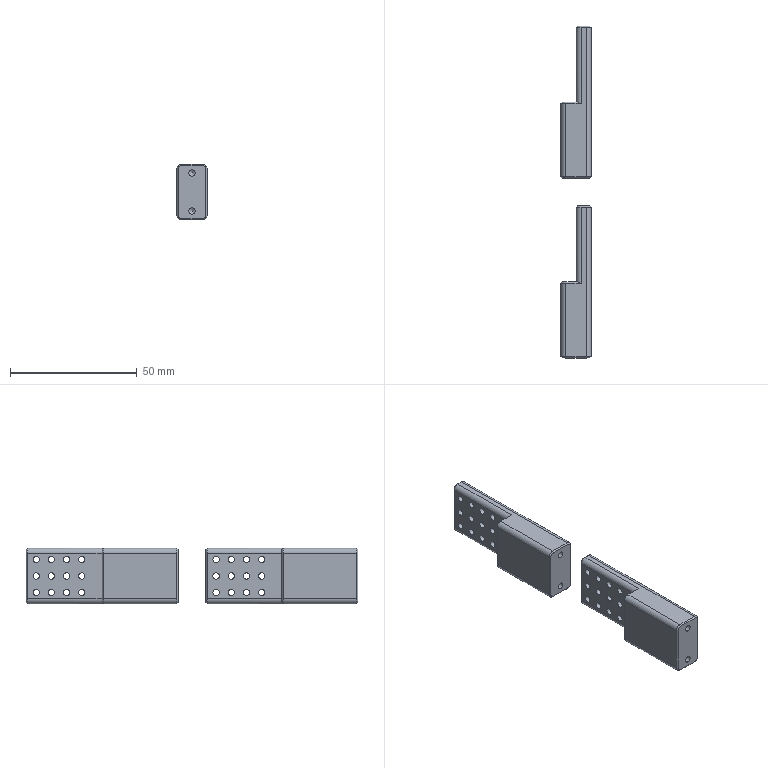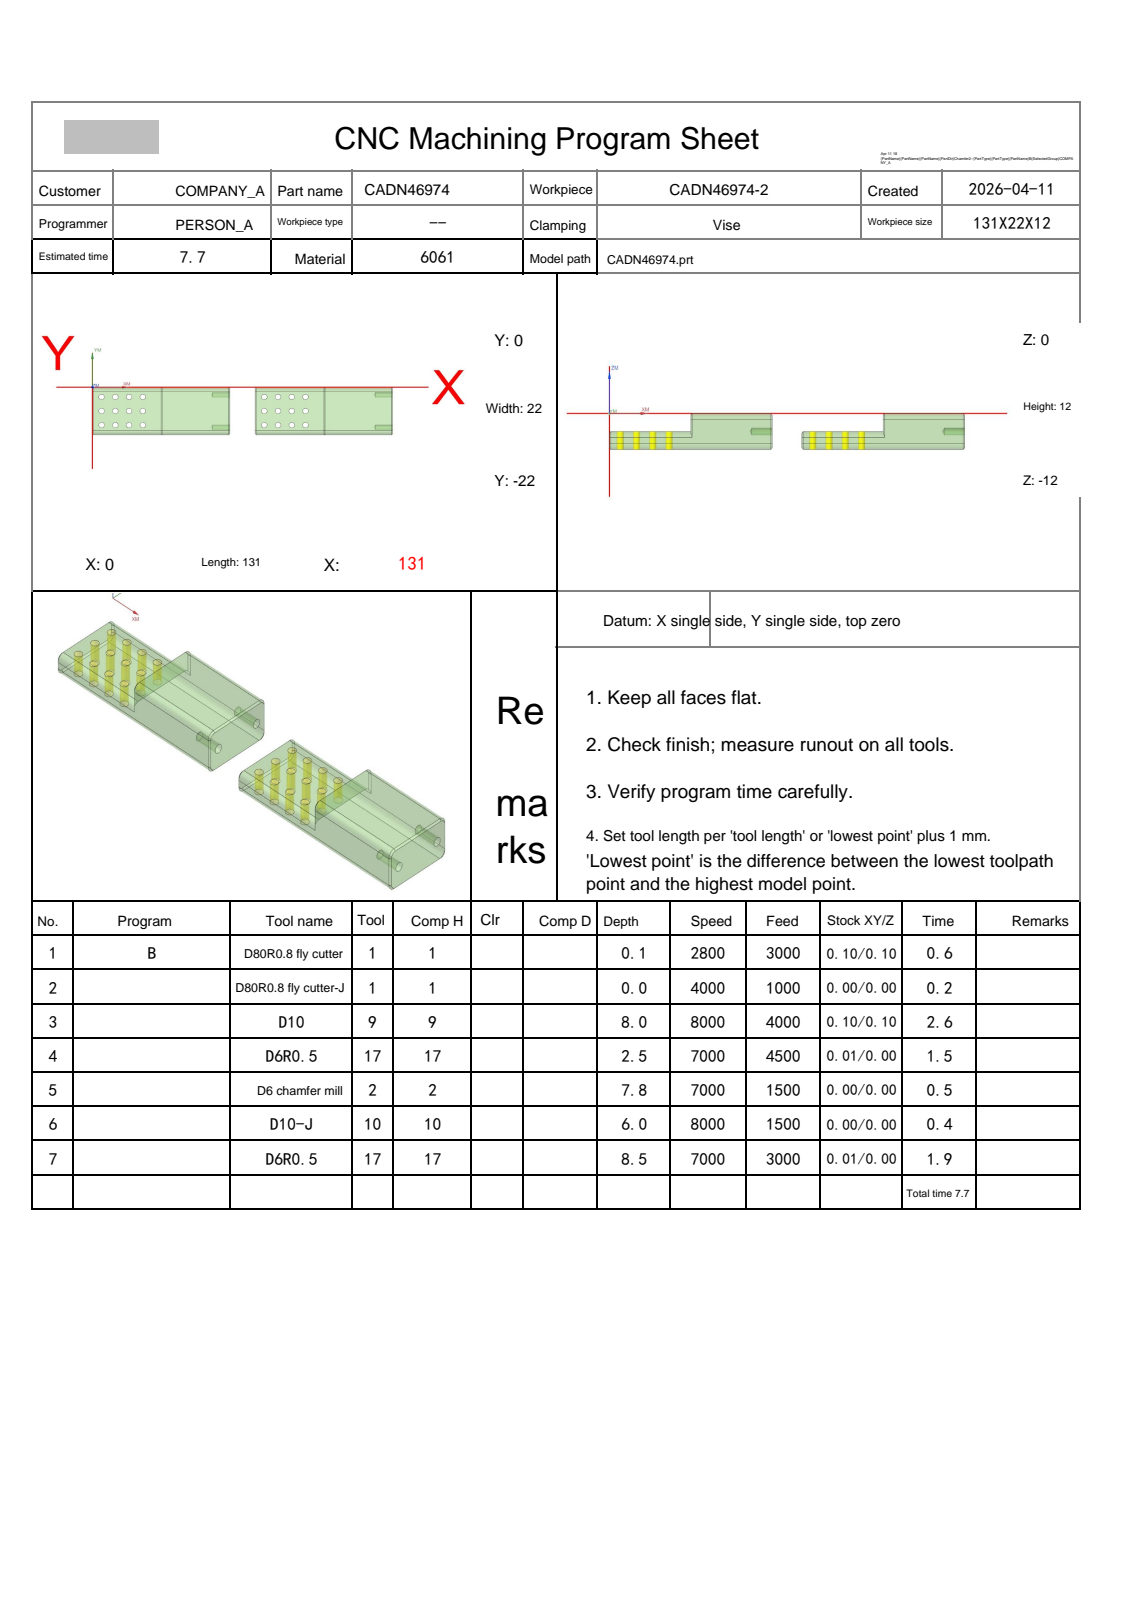NC program | NX | posted by the shop | part box 12 x 131 x 22 mm
Lines 1 to 2207 of 5054, first 1773 of 2205 lines:
%
O0001
(Machine time: 9.04 MIN)
(===Total Tool:5===)
(T1=D80R0.8 fly cutter D=80.  R=0.8  D-  H01 Z=0.    )
(T9=D10     D=10.  R=0.   D-  H09 Z=-8.   )
(T17=D6R0.5 D=6.   R=0.5  D-  H17 Z=-8.5  )
(T2=D6 chamfer mill   D=6.   R=0.   D-  H02 Z=-7.75 )
(T10=D10-J  D=10.  R=0.   D10 H10 Z=-6.   )
G80 G90 G17 G49 G40
G91 G28 Z0
M01
N1 T01 M06
(D80R0.8 fly cutter  D=80. R=0.8 H=01 ce=0.10 di=0.10)
G00 G90 G54 X183.097 Y-11. M03 S2800
G43 H01 Z20.
M08
Z4.517
G01 Z2.517 F3000.
X171.097
X-40.097
X-52.097
Z4.517
G00 X183.097
Z4.033
G01 Z2.033
X171.097
X-40.097
X-52.097
Z4.033
G00 X183.097
Z3.55
G01 Z1.55
X171.097
X-40.097
X-52.097
Z3.55
G00 X183.097
Z3.067
G01 Z1.067
X171.097
X-40.097
X-52.097
Z3.067
G00 Z20.
X183.097
Z2.583
G01 Z.583
X171.097
X-40.097
X-52.097
Z2.583
G00 Z20.
X183.097
Z2.1
G01 Z.1
X171.097
X-40.097
X-52.097
Z2.1
G00 Z20.
G91 G28 Z0.0
M05
M09
G91 G28 Z0.0
M01
N2 T01 M06
(D80R0.8 fly cutter-J  D=80. R=0.8 H=01 ce=0.00 di=0.00)
G00 G90 G54 X182.999 Y-11. M03 S4000
G43 H01 Z20.
M08
Z2.
G01 Z0.0 F1000.
X170.999
X-39.999
X-51.999
Z2.
G00 Z20.
G91 G28 Z0.0
M05
M09
G91 G28 Z0.0
M01
N3 T09 M06
(D10  D=10. R=0. H=09 ce=0.10 di=0.10)
G00 G90 G54 X18.201 Y-34.02 M03 S8000
G43 H09 Z12.8
M08
Z.708
G01 Z-.492 F4000.
Y-31.
G03 X11.201 Y-24. I-7. J0.0
G01 X4.502
X-1.996
X-1.999
G02 X-2.498 Y-23.507 I0.0 J.499
G01 X-2.5 Y1.507
G02 X-1.999 Y2.001 I.501 J-.006
G01 X-1.964 Y2.
X24.507
G02 X25.997 Y4.005 I7.492 J-4.012
X27.326 Y5.02 I4.489 J-4.5
G01 X58.797
X59.246
X59.378 Y5.022
G02 X63.361 Y3.238 I0.0 J-5.341
X64.059 Y2. I-8.104 J-5.382
X64.589 Y.608 I-8.801 J-4.144
G01 X64.591 Y.601
G03 X64.044 Y1.653 I-6.299 J-2.603
G01 X63.713 Y2.198
G03 X59.5 Y4.461 I-4.266 J-2.888
G01 X30.486
G03 X26.985 Y3.014 I0.0 J-4.956
X24.9 Y-2.001 I5.013 J-5.025
G01 Y-19.999
Y-20.028
G03 X26.176 Y-24.037 I6.936 J0.0
G01 X26.539 Y-24.526
G03 X30.5 Y-26.461 I4.015 J3.195
G01 X59.5
G03 X63.713 Y-24.198 I-.053 J5.151
X64.59 Y-22.581 I-6.897 J4.786
G01 X64.588 Y-22.587
X64.53 Y-22.798
X64.239 Y-23.627
G02 X64.095 Y-24. I-4.741 J1.615
X59.5 Y-27.02 I-4.597 J1.988
G01 X30.366
X29.131
X28.858
X27.348
G02 X25.416 Y-25.361 I3.208 J5.689
G01 X25.034 Y-24.847
G02 X24.507 Y-24. I6.803 J4.819
G01 X6.201
G02 X5.201 Y-23. I0.0 J1.
G01 X5.202 Y-22.95
X5.461 Y-17.759
X5.463 Y-17.709
G03 X4.982 Y-16.855 I-1. J0.0
G02 X4.501 Y-16.002 I.519 J.855
G01 Y-5.998
G02 X5.498 Y-5. I1. J-.002
G01 X16.903
G02 X17.9 Y-5.998 I-.002 J-1.
G01 Y-16.002
G02 X16.903 Y-17. I-1. J.002
G01 X9.643
G02 X8.743 Y-16.1 I0.0 J.9
G01 X8.744 Y-16.059
X9. Y-10.515
X9.001 Y-10.485
G02 X9.999 Y-9.5 I1. J-.015
G01 X12.403
G02 X13.4 Y-10.498 I-.002 J-1.
G01 Y-11.502
G02 X12.403 Y-12.5 I-1. J.002
G01 X9.999
G02 X9.433 Y-12.323 I.002 J1.
X9.108 Y-11.949 I.568 J.823
G03 X2.855 Y-8.096 I-6.253 J-3.146
X-.292 Y-8.843 I0.0 J-7.
G01 X-11.991 Y-14.729
Z.708
G00 Z3.
G01 X18.201 Y-34.18 F6000.
G00 Z.217
G01 Z-.983 F4000.
Y-31.
G03 X11.201 Y-24. I-7. J0.0
G01 X4.502
X-1.996
X-1.999
G02 X-2.498 Y-23.507 I0.0 J.499
G01 X-2.5 Y1.507
G02 X-1.999 Y2.001 I.501 J-.006
G01 X-1.964 Y2.
X24.18
G02 X25.066 Y3.361 I5.999 J-2.937
X26.976 Y5.18 I5.552 J-3.917
G01 X58.797
X59.243
X59.376 Y5.182
G02 X63.492 Y3.331 I0.0 J-5.501
X64.19 Y2.098 I-8.234 J-5.475
G01 X64.136 Y2.058
X64.082 Y2.13
G03 X63.042 Y3.398 I-6.938 J-4.629
X59.5 Y4.837 I-3.583 J-3.74
G01 X30.5
G03 X26.176 Y2.505 I.119 J-5.394
X24.9 Y-.898 I4.003 J-3.442
G01 Y-21.102
G03 X26.176 Y-24.505 I5.279 J.039
X30.5 Y-26.837 I4.442 J3.061
G01 X59.507
G03 X63.003 Y-25.429 I0.0 J5.044
X64.082 Y-24.13 I-5.234 J5.443
G01 X64.136 Y-24.058
X64.218 Y-24.118
G02 X59.5 Y-27.18 I-4.72 J2.106
G01 X30.366
X29.131
X28.858
X26.976
G02 X25.066 Y-25.361 I3.642 J5.736
X24.18 Y-24. I5.113 J4.298
G01 X6.201
G02 X5.201 Y-23. I0.0 J1.
G01 X5.202 Y-22.95
X5.461 Y-17.759
X5.462 Y-17.709
G03 X4.982 Y-16.855 I-1. J0.0
G02 X4.501 Y-16.002 I.519 J.855
G01 Y-5.998
G02 X5.498 Y-5. I1. J-.002
G01 X16.902
G02 X17.9 Y-5.998 I-.002 J-1.
G01 Y-16.002
G02 X16.902 Y-17. I-1. J.002
G01 X9.643
G02 X8.743 Y-16.1 I0.0 J.9
G01 X8.744 Y-16.059
X9. Y-10.515
X9.001 Y-10.485
G02 X9.999 Y-9.5 I1. J-.015
G01 X12.402
G02 X13.4 Y-10.498 I-.002 J-1.
G01 Y-11.502
G02 X12.402 Y-12.5 I-1. J.002
G01 X9.999
G02 X9.433 Y-12.323 I.002 J1.
X9.108 Y-11.949 I.568 J.823
G03 X2.855 Y-8.095 I-6.253 J-3.146
X-.291 Y-8.842 I0.0 J-7.
G01 X-12.151 Y-14.809
Z.217
G00 Z2.508
G01 X18.201 Y-34.18 F6000.
G00 Z-.275
G01 Z-1.475 F4000.
Y-31.
G03 X11.201 Y-24. I-7. J0.0
G01 X4.502
X-1.996
X-1.999
G02 X-2.498 Y-23.507 I0.0 J.499
G01 X-2.5 Y1.507
G02 X-1.999 Y2.001 I.501 J-.006
G01 X-1.964 Y2.
X24.052
G02 X25.413 Y3.995 I6.003 J-2.634
X26.688 Y5.18 I5.194 J-4.31
G01 X58.797
X59.243
X59.376 Y5.182
G02 X63.492 Y3.331 I0.0 J-5.501
X63.759 Y2.906 I-8.234 J-5.475
G01 X63.73 Y2.879
X63.222 Y3.398
G03 X59.5 Y5.033 I-3.748 J-3.477
G01 X30.5
G03 X26.45 Y3.052 I.107 J-5.348
X24.9 Y-.591 I3.605 J-3.685
G01 Y-21.409
G03 X26.45 Y-25.052 I5.155 J.043
X30.5 Y-27.033 I4.153 J3.358
G01 X59.5
G03 X63.222 Y-25.398 I-.025 J5.112
G01 X63.717 Y-24.892
X63.76 Y-24.934
G02 X59.5 Y-27.18 I-4.263 J2.922
G01 X30.366
X29.131
X28.858
X26.687
G02 X25.413 Y-25.995 I3.916 J5.486
X24.052 Y-24. I4.642 J4.629
G01 X6.201
G02 X5.201 Y-23. I0.0 J1.
G01 X5.202 Y-22.95
X5.461 Y-17.759
X5.462 Y-17.709
G03 X4.982 Y-16.855 I-1. J0.0
G02 X4.501 Y-16.002 I.519 J.855
G01 Y-5.998
G02 X5.498 Y-5. I1. J-.002
G01 X16.902
G02 X17.9 Y-5.998 I-.002 J-1.
G01 Y-16.002
G02 X16.902 Y-17. I-1. J.002
G01 X9.643
G02 X8.743 Y-16.1 I0.0 J.9
G01 X8.744 Y-16.059
X9. Y-10.515
X9.001 Y-10.485
G02 X9.998 Y-9.5 I1. J-.015
G01 X12.403
G02 X13.4 Y-10.497 I-.003 J-1.
G01 Y-11.503
G02 X12.403 Y-12.5 I-1. J.003
G01 X9.999
G02 X9.433 Y-12.323 I.003 J1.
X9.108 Y-11.949 I.568 J.823
G03 X2.855 Y-8.095 I-6.253 J-3.146
X-.291 Y-8.842 I0.0 J-7.
G01 X-12.151 Y-14.809
Z-.275
G00 Z2.017
G01 X18.201 Y-34.18 F6000.
G00 Z-.767
G01 Z-1.967 F4000.
Y-31.
G03 X11.201 Y-24. I-7. J0.0
G01 X4.502
X-1.996
X-1.999
G02 X-2.498 Y-23.507 I0.0 J.499
G01 X-2.5 Y1.507
G02 X-1.999 Y2.001 I.501 J-.006
G01 X-1.964 Y2.
X24.002
G02 X25.363 Y4.052 I6.008 J-2.508
X26.581 Y5.18 I5.495 J-4.707
G01 X58.797
X59.243
X59.374 Y5.182
G02 X63.499 Y3.32 I0.0 J-5.501
G01 X63.451 Y3.269
X63.342 Y3.368
G03 X59.534 Y5.1 I-3.862 J-3.441
G01 X30.404
G03 X28.858 Y4.826 I0.0 J-4.511
X26.396 Y3.104 I2.001 J-5.481
X24.9 Y-.501 I3.615 J-3.612
G01 Y-21.509
G03 X26.071 Y-24.741 I5.044 J0.0
X27.331 Y-25.981 I6.952 J5.801
X30.494 Y-27.1 I3.164 J3.913
G01 X59.534
X59.602
G03 X62.637 Y-26.009 I0.0 J4.763
G01 X62.989 Y-25.709
X63.229 Y-25.478
X63.282 Y-25.532
G02 X59.5 Y-27.18 I-3.784 J3.52
G01 X30.366
X29.131
X28.858
X26.591
X26.451 Y-27.07
G02 X24.996 Y-25.638 I6.573 J8.13
X24.001 Y-24. I4.947 J4.128
G01 X6.201
G02 X5.201 Y-23. I0.0 J1.
G01 X5.202 Y-22.95
X5.461 Y-17.758
X5.462 Y-17.709
G03 X4.982 Y-16.855 I-1. J0.0
G02 X4.501 Y-16.003 I.519 J.855
G01 Y-5.997
G02 X5.498 Y-5. I1. J-.002
G01 X16.903
G02 X17.9 Y-5.997 I-.003 J-1.
G01 Y-16.003
G02 X16.903 Y-17. I-1. J.003
G01 X9.643
G02 X8.743 Y-16.1 I0.0 J.9
G01 X8.744 Y-16.059
X9. Y-10.515
X9.001 Y-10.485
G02 X9.998 Y-9.5 I1. J-.015
G01 X12.403
G02 X13.4 Y-10.497 I-.003 J-1.
G01 Y-11.503
G02 X12.403 Y-12.5 I-1. J.003
G01 X9.998
G02 X9.433 Y-12.323 I.003 J1.
X9.108 Y-11.949 I.568 J.823
G03 X2.855 Y-8.095 I-6.253 J-3.146
X-.291 Y-8.842 I0.0 J-7.
G01 X-12.151 Y-14.809
Z-.767
G00 Z1.525
G01 X18.201 Y-34.18 F6000.
G00 Z-1.258
G01 Z-2.458 F4000.
Y-31.
G03 X11.201 Y-24. I-7. J0.0
G01 X4.502
X-1.996
X-1.999
G02 X-2.498 Y-23.507 I0.0 J.499
G01 X-2.5 Y1.507
G02 X-1.999 Y2.001 I.501 J-.006
G01 X-1.964 Y2.
X24.
G02 X25.388 Y4.08 I6. J-2.5
X26.384 Y5.03 I5.47 J-4.735
X26.574 Y5.18 I4.116 J-5.03
G01 X30.529
Y5.1
X30.404
X30.401
G03 X28.896 Y4.841 I0.0 J-4.512
X27.26 Y3.939 I1.604 J-4.841
X26.394 Y3.106 I3.59 J-4.603
X24.9 Y-.5 I3.606 J-3.606
G01 Y-21.509
G03 X25.171 Y-23.142 I5.044 J0.0
X26.386 Y-25.098 I4.829 J1.642
X26.894 Y-25.606 I6.653 J6.144
X30.5 Y-27.1 I3.606 J3.606
G01 X30.529
Y-27.18
X30.366
X29.131
X28.858
X26.574
G02 X25.892 Y-26.585 I3.926 J5.18
X25.376 Y-26.068 I7.131 J7.645
X24. Y-24. I4.624 J4.568
G01 X6.201
G02 X5.201 Y-23. I0.0 J1.
G01 X5.202 Y-22.95
X5.461 Y-17.758
X5.462 Y-17.709
G03 X4.982 Y-16.855 I-1. J0.0
G02 X4.501 Y-16.003 I.519 J.855
G01 Y-5.997
G02 X5.498 Y-5. I1. J-.003
G01 X16.903
G02 X17.9 Y-5.997 I-.003 J-1.
G01 Y-16.003
G02 X16.903 Y-17. I-1. J.003
G01 X9.643
G02 X8.743 Y-16.1 I0.0 J.9
G01 X8.744 Y-16.059
X9. Y-10.515
X9.001 Y-10.485
G02 X9.998 Y-9.5 I1. J-.015
G01 X12.403
G02 X13.4 Y-10.497 I-.003 J-1.
G01 Y-11.503
G02 X12.403 Y-12.5 I-1. J.003
G01 X9.998
G02 X9.433 Y-12.323 I.003 J1.
X9.108 Y-11.949 I.568 J.823
G03 X2.855 Y-8.095 I-6.253 J-3.146
X-.291 Y-8.842 I0.0 J-7.
G01 X-12.151 Y-14.809
Z-1.258
G00 Z1.033
G01 X18.201 Y-34.18 F6000.
G00 Z-1.75
G01 Z-2.95 F4000.
Y-31.
G03 X11.201 Y-24. I-7. J0.0
G01 X4.502
X-1.996
X-1.999
G02 X-2.498 Y-23.507 I0.0 J.499
G01 X-2.5 Y1.507
G02 X-1.999 Y2.001 I.501 J-.006
G01 X-1.964 Y2.
X24.
G02 X25.388 Y4.08 I6. J-2.5
X26.384 Y5.03 I5.47 J-4.735
X26.574 Y5.18 I4.116 J-5.03
G01 X30.524
Y5.1
X30.404
G03 X28.942 Y4.856 I0.0 J-4.511
X27.26 Y3.939 I1.558 J-4.856
X26.394 Y3.106 I3.59 J-4.603
X24.9 Y-.5 I3.606 J-3.606
G01 Y-21.509
G03 X25.171 Y-23.141 I5.044 J0.0
X26.386 Y-25.098 I4.829 J1.641
X26.894 Y-25.606 I6.653 J6.144
X30.5 Y-27.1 I3.606 J3.606
G01 X30.524
Y-27.18
X30.366
X29.131
X28.858
X26.574
G02 X25.892 Y-26.585 I3.926 J5.18
X25.376 Y-26.068 I7.131 J7.645
X24. Y-24. I4.624 J4.568
G01 X6.201
G02 X5.201 Y-23. I0.0 J1.
G01 X5.202 Y-22.95
X5.461 Y-17.758
X5.462 Y-17.709
G03 X4.982 Y-16.854 I-1. J0.0
G02 X4.501 Y-16.003 I.52 J.854
G01 Y-5.997
G02 X5.498 Y-5. I1. J-.003
G01 X16.903
G02 X17.9 Y-5.997 I-.003 J-1.
G01 Y-16.003
G02 X16.903 Y-17. I-1. J.003
G01 X9.643
G02 X8.743 Y-16.1 I0.0 J.9
G01 X8.744 Y-16.059
X9. Y-10.515
X9.001 Y-10.485
G02 X9.998 Y-9.5 I1. J-.015
G01 X12.403
G02 X13.4 Y-10.497 I-.003 J-1.
G01 Y-11.503
G02 X12.403 Y-12.5 I-1. J.003
G01 X9.998
G02 X9.433 Y-12.323 I.003 J1.
X9.108 Y-11.949 I.568 J.823
G03 X2.855 Y-8.095 I-6.253 J-3.146
X-.291 Y-8.842 I0.0 J-7.
G01 X-12.151 Y-14.809
Z-1.75
G00 Z.542
G01 X18.201 Y-34.18 F6000.
G00 Z-2.242
G01 Z-3.442 F4000.
Y-31.
G03 X11.201 Y-24. I-7. J0.0
G01 X4.502
X-1.996
X-1.999
G02 X-2.498 Y-23.507 I0.0 J.499
G01 X-2.5 Y1.507
G02 X-1.999 Y2.001 I.501 J-.006
G01 X-1.964 Y2.
X24.
G02 X25.388 Y4.08 I6. J-2.5
X26.384 Y5.03 I5.47 J-4.735
X26.574 Y5.18 I4.116 J-5.03
G01 X30.52
Y5.1
X30.404
G03 X28.942 Y4.856 I0.0 J-4.511
X27.26 Y3.939 I1.558 J-4.856
X26.394 Y3.106 I3.59 J-4.603
X24.9 Y-.5 I3.606 J-3.606
G01 Y-21.509
G03 X25.171 Y-23.141 I5.044 J0.0
X26.386 Y-25.098 I4.829 J1.641
X26.621 Y-25.342 I6.638 J6.158
X26.894 Y-25.606 I6.431 J6.376
X30.5 Y-27.1 I3.606 J3.606
G01 X30.52
Y-27.18
X30.366
X29.131
X28.858
X26.574
G02 X25.892 Y-26.585 I3.926 J5.18
X25.376 Y-26.068 I7.131 J7.645
X24. Y-24. I4.624 J4.568
G01 X6.201
G02 X5.201 Y-23. I0.0 J1.
G01 X5.202 Y-22.95
X5.461 Y-17.758
X5.462 Y-17.709
G03 X4.982 Y-16.854 I-1. J0.0
G02 X4.501 Y-16.003 I.52 J.854
G01 Y-5.997
G02 X5.498 Y-5. I1. J-.003
G01 X16.903
G02 X17.9 Y-5.997 I-.003 J-1.
G01 Y-16.003
G02 X16.903 Y-17. I-1. J.003
G01 X9.643
G02 X8.743 Y-16.1 I0.0 J.9
G01 X8.744 Y-16.059
X9. Y-10.514
X9.001 Y-10.484
G02 X9.998 Y-9.5 I1. J-.016
G01 X12.403
G02 X13.4 Y-10.497 I-.003 J-1.
G01 Y-11.503
G02 X12.403 Y-12.5 I-1. J.003
G01 X9.998
G02 X9.433 Y-12.323 I.003 J1.
X9.108 Y-11.949 I.568 J.823
G03 X2.855 Y-8.095 I-6.253 J-3.146
X-.291 Y-8.842 I0.0 J-7.
G01 X-12.151 Y-14.809
Z-2.242
G00 Z.05
G01 X18.201 Y-34.18 F6000.
G00 Z-2.733
G01 Z-3.933 F4000.
Y-31.
G03 X11.201 Y-24. I-7. J0.0
G01 X4.502
X-1.996
X-1.999
G02 X-2.498 Y-23.507 I0.0 J.499
G01 X-2.5 Y1.507
G02 X-1.999 Y2.001 I.501 J-.006
G01 X-1.964 Y2.
X24.
G02 X25.388 Y4.08 I6. J-2.5
X26.384 Y5.03 I5.47 J-4.735
X26.574 Y5.18 I4.116 J-5.03
G01 X30.515
Y5.1
X30.293 Y5.098
G03 X28.942 Y4.856 I.111 J-4.51
X27.26 Y3.939 I1.558 J-4.856
X26.394 Y3.106 I3.59 J-4.603
X24.9 Y-.5 I3.606 J-3.606
G01 Y-21.509
G03 X25.171 Y-23.141 I5.044 J0.0
X26.404 Y-25.118 I4.83 J1.64
X26.894 Y-25.606 I6.635 J6.164
X30.5 Y-27.1 I3.606 J3.606
G01 X30.515
Y-27.18
X30.366
X29.131
X28.858
X26.574
G02 X25.892 Y-26.585 I3.926 J5.18
X25.376 Y-26.068 I7.131 J7.645
X24. Y-24. I4.624 J4.568
G01 X6.201
G02 X5.201 Y-23. I0.0 J1.
G01 X5.202 Y-22.95
X5.46 Y-17.758
X5.462 Y-17.708
G03 X4.982 Y-16.854 I-1. J0.0
G02 X4.501 Y-16.003 I.52 J.854
G01 Y-5.997
G02 X5.497 Y-5. I1. J-.003
G01 X16.903
G02 X17.9 Y-5.997 I-.003 J-1.
G01 Y-16.003
G02 X16.903 Y-17. I-1. J.003
G01 X9.643
G02 X8.743 Y-16.1 I0.0 J.9
G01 X8.744 Y-16.059
X9. Y-10.514
X9.001 Y-10.484
G02 X9.998 Y-9.5 I1. J-.016
G01 X12.403
G02 X13.4 Y-10.497 I-.003 J-1.
G01 Y-11.503
G02 X12.403 Y-12.5 I-1. J.003
G01 X9.998
G02 X9.433 Y-12.323 I.003 J1.
X9.108 Y-11.949 I.568 J.823
G03 X2.855 Y-8.095 I-6.253 J-3.146
X-.291 Y-8.842 I0.0 J-7.
G01 X-12.151 Y-14.809
Z-2.733
G00 Z-.442
G01 X18.201 Y-34.18 F6000.
G00 Z-3.225
G01 Z-4.425 F4000.
Y-31.
G03 X11.201 Y-24. I-7. J0.0
G01 X4.502
X-1.996
X-1.999
G02 X-2.498 Y-23.507 I0.0 J.499
G01 X-2.5 Y1.507
G02 X-1.999 Y2.001 I.501 J-.006
G01 X-1.964 Y2.
X24.
G02 X25.388 Y4.08 I6. J-2.5
X26.384 Y5.03 I5.47 J-4.735
X26.574 Y5.18 I4.116 J-5.03
G01 X30.511
Y5.1
X30.404
G03 X28.942 Y4.856 I0.0 J-4.511
X27.26 Y3.939 I1.558 J-4.856
X26.394 Y3.106 I3.59 J-4.603
X24.9 Y-.5 I3.606 J-3.606
G01 Y-21.509
G03 X25.171 Y-23.141 I5.044 J0.0
X26.386 Y-25.098 I4.829 J1.641
X26.894 Y-25.606 I6.653 J6.144
X30.5 Y-27.1 I3.606 J3.606
G01 X30.511
Y-27.18
X30.366
X29.131
X28.858
X26.574
G02 X25.892 Y-26.585 I3.926 J5.18
X25.376 Y-26.068 I7.131 J7.645
X24. Y-24. I4.624 J4.568
G01 X6.201
G02 X5.201 Y-23. I0.0 J1.
G01 X5.202 Y-22.95
X5.46 Y-17.758
X5.462 Y-17.708
G03 X4.982 Y-16.854 I-1. J0.0
G02 X4.501 Y-16.004 I.52 J.854
G01 Y-5.997
G02 X5.497 Y-5. I1. J-.003
G01 X16.903
G02 X17.9 Y-5.997 I-.003 J-1.
G01 Y-16.003
G02 X16.903 Y-17. I-1. J.003
G01 X9.643
G02 X8.743 Y-16.1 I0.0 J.9
G01 X8.744 Y-16.059
X9. Y-10.514
X9.001 Y-10.484
G02 X9.997 Y-9.5 I1. J-.016
G01 X12.404
G02 X13.4 Y-10.496 I-.004 J-1.
G01 Y-11.504
G02 X12.404 Y-12.5 I-1. J.004
G01 X9.998
G02 X9.433 Y-12.323 I.004 J1.
X9.108 Y-11.949 I.568 J.823
G03 X2.855 Y-8.095 I-6.253 J-3.146
X-.291 Y-8.842 I0.0 J-7.
G01 X-12.151 Y-14.809
Z-3.225
G00 Z-.933
G01 X18.201 Y-34.18 F6000.
G00 Z-3.717
G01 Z-4.917 F4000.
Y-31.
G03 X11.201 Y-24. I-7. J0.0
G01 X4.502
X-1.996
X-1.999
G02 X-2.498 Y-23.507 I0.0 J.499
G01 X-2.5 Y1.507
G02 X-1.999 Y2.001 I.501 J-.006
G01 X-1.964 Y2.
X24.
G02 X25.388 Y4.08 I6. J-2.5
X26.384 Y5.03 I5.47 J-4.735
X26.574 Y5.18 I4.116 J-5.03
G01 X30.506
Y5.1
X30.404
G03 X28.942 Y4.856 I0.0 J-4.511
X27.26 Y3.939 I1.558 J-4.856
X26.394 Y3.106 I3.59 J-4.603
X24.9 Y-.5 I3.606 J-3.606
G01 Y-21.509
G03 X25.171 Y-23.141 I5.044 J0.0
X26.386 Y-25.098 I4.829 J1.641
X26.894 Y-25.606 I6.653 J6.144
X30.5 Y-27.1 I3.606 J3.606
G01 X30.506
Y-27.18
X30.366
X29.131
X28.858
X26.574
G02 X25.892 Y-26.585 I3.926 J5.18
X25.376 Y-26.068 I7.131 J7.645
X24. Y-24. I4.624 J4.568
G01 X6.201
G02 X5.201 Y-23. I0.0 J1.
G01 X5.202 Y-22.95
X5.46 Y-17.758
X5.461 Y-17.708
G03 X4.982 Y-16.854 I-1. J0.0
G02 X4.501 Y-16.004 I.52 J.854
G01 Y-5.996
G02 X5.497 Y-5. I1. J-.003
G01 X16.904
G02 X17.9 Y-5.996 I-.004 J-1.
G01 Y-16.004
G02 X16.904 Y-17. I-1. J.004
G01 X9.643
G02 X8.743 Y-16.1 I0.0 J.9
G01 X8.744 Y-16.059
X9. Y-10.514
X9.001 Y-10.484
G02 X9.997 Y-9.5 I1. J-.016
G01 X12.404
G02 X13.4 Y-10.496 I-.004 J-1.
G01 Y-11.504
G02 X12.404 Y-12.5 I-1. J.004
G01 X9.997
G02 X9.433 Y-12.323 I.004 J1.
X9.108 Y-11.949 I.568 J.823
G03 X2.855 Y-8.095 I-6.253 J-3.146
X-.291 Y-8.842 I0.0 J-7.
G01 X-12.151 Y-14.809
Z-3.717
G00 Z-1.425
G01 X18.201 Y-34.18 F6000.
G00 Z-4.208
G01 Z-5.408 F4000.
Y-31.
G03 X11.201 Y-24. I-7. J0.0
G01 X4.502
X-1.996
X-1.999
G02 X-2.498 Y-23.507 I0.0 J.499
G01 X-2.5 Y1.507
G02 X-1.999 Y2.001 I.501 J-.006
G01 X-1.964 Y2.
X24.
G02 X25.388 Y4.08 I6. J-2.5
X26.384 Y5.03 I5.47 J-4.735
X26.574 Y5.18 I4.116 J-5.03
G01 X30.502
Y5.1
X30.404
G03 X28.942 Y4.856 I0.0 J-4.511
X27.26 Y3.939 I1.558 J-4.856
X26.394 Y3.106 I3.59 J-4.603
X24.9 Y-.5 I3.606 J-3.606
G01 Y-21.509
G03 X25.171 Y-23.141 I5.044 J0.0
X26.386 Y-25.098 I4.829 J1.641
X26.894 Y-25.606 I6.653 J6.144
X30.5 Y-27.1 I3.606 J3.606
G01 X30.502
Y-27.18
X30.366
X29.131
X28.858
X26.574
G02 X25.892 Y-26.585 I3.926 J5.18
X25.376 Y-26.068 I7.131 J7.645
X24. Y-24. I4.624 J4.568
G01 X6.201
G02 X5.201 Y-23. I0.0 J1.
G01 X5.202 Y-22.95
X5.46 Y-17.758
X5.461 Y-17.708
G03 X4.982 Y-16.854 I-1. J0.0
G02 X4.501 Y-16.004 I.52 J.854
G01 Y-5.996
G02 X5.497 Y-5. I1. J-.004
G01 X16.904
G02 X17.9 Y-5.996 I-.004 J-1.
G01 Y-16.004
G02 X16.904 Y-17. I-1. J.004
G01 X9.643
G02 X8.743 Y-16.1 I0.0 J.9
G01 X8.744 Y-16.059
X9. Y-10.514
X9.001 Y-10.484
G02 X9.997 Y-9.5 I1. J-.016
G01 X12.404
G02 X13.4 Y-10.496 I-.004 J-1.
G01 Y-11.504
G02 X12.404 Y-12.5 I-1. J.004
G01 X9.997
G02 X9.433 Y-12.323 I.004 J1.
X9.108 Y-11.949 I.568 J.823
G03 X2.855 Y-8.095 I-6.253 J-3.146
X-.291 Y-8.842 I0.0 J-7.
G01 X-12.151 Y-14.809
Z-4.208
G00 Z-1.917
G01 X18.201 Y-34.18 F6000.
G00 Z-4.7
G01 Z-5.9 F4000.
Y-31.
G03 X11.201 Y-24. I-7. J0.0
G01 X4.502
X-1.996
X-1.999
G02 X-2.498 Y-23.507 I0.0 J.499
G01 X-2.5 Y1.507
G02 X-1.999 Y2.001 I.501 J-.006
G01 X-1.964 Y2.
X24.
G02 X25.388 Y4.08 I6. J-2.5
X26.384 Y5.03 I5.47 J-4.735
X26.574 Y5.18 I4.116 J-5.03
G01 X30.496
X30.497 Y5.1
X30.404
G03 X28.942 Y4.856 I0.0 J-4.511
X27.26 Y3.939 I1.558 J-4.856
X26.394 Y3.106 I3.59 J-4.603
X24.9 Y-.5 I3.606 J-3.606
G01 Y-21.509
G03 X25.171 Y-23.141 I5.044 J0.0
X26.386 Y-25.098 I4.829 J1.641
X26.894 Y-25.606 I6.653 J6.144
X27.532 Y-26.147 I3.606 J3.606
X30.497 Y-27.1 I2.968 J4.147
G01 X30.496 Y-27.18
X30.366
X29.131
X28.858
X26.574
G02 X25.892 Y-26.585 I3.926 J5.18
X25.376 Y-26.068 I7.131 J7.645
X24. Y-24. I4.624 J4.568
G01 X6.201
G02 X5.201 Y-23. I0.0 J1.
G01 X5.202 Y-22.95
X5.46 Y-17.757
X5.461 Y-17.708
G03 X4.982 Y-16.854 I-1. J0.0
G02 X4.501 Y-16.004 I.52 J.854
G01 Y-5.996
G02 X5.497 Y-5. I1. J-.004
G01 X16.904
G02 X17.9 Y-5.996 I-.004 J-1.
G01 Y-16.004
G02 X16.904 Y-17. I-1. J.004
G01 X9.643
G02 X8.743 Y-16.1 I0.0 J.9
G01 X8.744 Y-16.059
X9. Y-10.513
X9.001 Y-10.484
G02 X9.997 Y-9.5 I1. J-.016
G01 X12.404
G02 X13.4 Y-10.496 I-.004 J-1.
G01 Y-11.504
G02 X12.404 Y-12.5 I-1. J.004
G01 X9.997
G02 X9.433 Y-12.323 I.004 J1.
X9.108 Y-11.949 I.568 J.823
G03 X2.855 Y-8.095 I-6.253 J-3.146
X-.291 Y-8.842 I0.0 J-7.
G01 X-12.151 Y-14.809
Z-4.7
G00 Z-2.408
G01 X22.824 Y-34.18 F6000.
G00 Z-5.12
G01 Z-6.32 F4000.
G03 X15.824 Y-27.18 I-7. J0.0
G01 X1.155
G02 X.743 Y-27.195 I-.412 J5.649
X-3.802 Y-24.911 I0.0 J5.664
X-5.141 Y-20.163 I9.855 J5.342
G01 X-5.151 Y-17.545
Y-2.711
G02 X-5.155 Y-2.395 I11.023 J.316
X-3.721 Y3.043 I11.027 J0.0
X.743 Y5.195 I4.464 J-3.552
X1.155 Y5.18 I0.0 J-5.705
G01 X30.493
Y5.1
X30.404
G03 X28.942 Y4.856 I0.0 J-4.511
X27.696 Y4.26 I1.558 J-4.856
G01 X.438
G03 X-3.549 Y2.221 I0.0 J-4.918
X-4.961 Y-2. I6.057 J-4.374
G01 Y-20.
G03 X-3.549 Y-24.221 I7.47 J.153
X.438 Y-26.26 I3.987 J2.879
G01 X27.696
G03 X30.493 Y-27.1 I2.804 J4.26
G01 Y-27.18
X30.366
X29.131
X28.858
X15.824
X15.324
G03 X8.324 Y-34.18 I0.0 J-7.
G01 Z-5.12
G00 Z-2.9
G01 X8.822 Y12.18 F6000.
G00 Z-5.54
G01 Z-6.74 F4000.
G03 X15.822 Y5.18 I7. J0.0
G01 X30.489
Y5.1
X30.404
G03 X28.942 Y4.856 I0.0 J-4.511
X28.473 Y4.68 I1.558 J-4.856
G01 X.5
G03 X-3.153 Y3.121 I0.0 J-5.058
X-4.39 Y1.404 I5.475 J-5.25
G01 X-4.47 Y1.433
G02 X-3.721 Y3.043 I10.34 J-3.833
X.743 Y5.195 I4.464 J-3.552
X1.155 Y5.18 I0.0 J-5.705
G01 X15.822
X16.322
G03 X23.322 Y12.18 I0.0 J7.
G01 Z-5.54
G00 Z-3.32
G01 X8.822 F6000.
G00 Z-5.96
G01 Z-7.16 F4000.
G03 X15.822 Y5.18 I7. J0.0
G01 X30.485
Y5.1
X30.404
G03 X29.16 Y4.925 I0.0 J-4.511
G01 X.496
G03 X-3.271 Y3.241 I0.0 J-5.056
G01 X-3.948 Y2.479
X-4.006 Y2.508
G02 X-3.721 Y3.043 I9.87 J-4.917
X.743 Y5.195 I4.464 J-3.552
X1.155 Y5.18 I0.0 J-5.705
G01 X15.822
X16.322
G03 X23.322 Y12.18 I0.0 J7.
G01 Z-5.96
G00 Z-3.74
G01 X8.822 F6000.
G00 Z-6.38
G01 Z-7.58 F4000.
G03 X15.822 Y5.18 I7. J0.0
G01 X30.481
Y5.1
X30.404
G03 X29.789 Y5.058 I0.0 J-4.511
G01 X.5
X-.635 Y4.913
G03 X-3.623 Y2.984 I1.25 J-5.214
G01 X-3.655 Y2.952
X-3.745 Y3.002
X-3.721 Y3.043
G02 X.743 Y5.195 I4.464 J-3.552
X1.155 Y5.18 I0.0 J-5.705
G01 X15.822
X16.322
G03 X23.322 Y12.18 I0.0 J7.
G01 Z-6.38
G00 Z-4.16
G01 X8.822 F6000.
G00 Z-6.8
G01 Z-8. F4000.
G03 X15.822 Y5.18 I7. J0.0
G01 X30.477
Y5.1
X.513
G03 X-3.316 Y3.396 I0.0 J-5.155
G01 X-3.368 Y3.446
G02 X.743 Y5.195 I4.111 J-3.955
X1.155 Y5.18 I0.0 J-5.705
G01 X15.822
X16.322
G03 X23.322 Y12.18 I0.0 J7.
G01 Z-6.8
G00 Z-2.9
G01 X22.822 Y-34.18 F6000.
G00 Z-5.54
G01 Z-6.74 F4000.
G03 X15.822 Y-27.18 I-7. J0.0
G01 X1.155
G02 X.743 Y-27.195 I-.412 J5.649
X-3.802 Y-24.911 I0.0 J5.664
X-4.47 Y-23.433 I9.855 J5.342
G01 X-4.39 Y-23.404
X-4.264 Y-23.653
X-3.659 Y-24.526
G03 X.5 Y-26.68 I4.193 J3.003
G01 X28.473
G03 X30.489 Y-27.1 I2.027 J4.68
G01 Y-27.18
X30.366
X29.131
X28.858
X15.822
X15.322
G03 X8.322 Y-34.18 I0.0 J-7.
G01 Z-5.54
G00 Z-3.32
G01 X22.822 F6000.
G00 Z-5.96
G01 Z-7.16 F4000.
G03 X15.822 Y-27.18 I-7. J0.0
G01 X1.155
G02 X.743 Y-27.195 I-.412 J5.649
X-3.802 Y-24.911 I0.0 J5.664
X-4.001 Y-24.525 I9.855 J5.342
G01 X-3.936 Y-24.493
X-3.269 Y-25.243
G03 X.493 Y-26.925 I3.763 J3.368
G01 X29.174
G03 X30.485 Y-27.1 I1.325 J4.925
G01 Y-27.18
X29.131
X28.858
X15.822
X15.322
G03 X8.322 Y-34.18 I0.0 J-7.
G01 Z-5.96
G00 Z-3.74
G01 X22.822 F6000.
G00 Z-6.38
G01 Z-7.58 F4000.
G03 X15.822 Y-27.18 I-7. J0.0
G01 X1.155
G02 X.742 Y-27.195 I-.413 J5.649
X-3.699 Y-25.046 I0.0 J5.664
G01 X-3.622 Y-24.985
G03 X-1.976 Y-26.402 I4.737 J3.838
X.5 Y-27.058 I2.675 J5.101
G01 X29.844
G03 X30.481 Y-27.1 I.656 J5.058
G01 X30.477 Y-27.18
X29.131
X28.858
X15.822
X15.322
G03 X8.322 Y-34.18 I0.0 J-7.
G01 Z-6.38
G00 Z-4.16
G01 X22.822 F6000.
G00 Z-6.8
G01 Z-8. F4000.
G03 X15.822 Y-27.18 I-7. J0.0
G01 X1.155
G02 X.742 Y-27.195 I-.413 J5.649
X-3.36 Y-25.437 I0.0 J5.664
G01 X-3.316 Y-25.396
G03 X.513 Y-27.1 I3.829 J3.45
G01 X30.477
Y-27.18
X29.131
X28.858
X15.822
X15.322
G03 X8.322 Y-34.18 I0.0 J-7.
G01 Z-6.8
G00 Z3.
G01 X87.955 Y-34.02 F6000.
G00 Z.708
G01 Z-.492 F4000.
Y-31.
G03 X80.955 Y-24. I-7. J0.0
G01 X66.921
G02 X66.019 Y-20.161 I9.503 J4.259
G01 X66.009 Y-18.417
Y-2.708
G02 X66.005 Y-2.398 I11.084 J.31
X66.761 Y1.627 I11.088 J0.0
X66.907 Y2. I5.048 J-1.752
G01 X95.506
G02 X96.627 Y3.634 I7.666 J-4.055
X98.35 Y5.02 I4.956 J-4.399
G01 X128.06
X130.736 Y5.014
X131.617 Y4.894
X132.497 Y4.605
X133.246 Y4.202
X133.373 Y4.116
X134.259 Y3.34
X134.554 Y3.036
G02 X135.519 Y.77 I-9.802 J-5.516
G03 X134.465 Y2.526 I-7.431 J-3.27
X130.5 Y4.461 I-4.048 J-3.264
G01 X101.5
G03 X97.674 Y2.705 I.082 J-5.226
X95.9 Y-2.001 I5.499 J-4.759
G01 Y-19.999
Y-20.075
G03 X96.942 Y-23.653 I6.661 J0.0
G01 X97.517 Y-24.526
G03 X101.5 Y-26.461 I4.069 J3.307
G01 X130.5
G03 X134.316 Y-24.701 I-.07 J5.169
X135.596 Y-22.593 I-6.12 J5.157
G01 X135.548 Y-22.755
X135.227 Y-23.624
X135.137 Y-23.843
X134.838 Y-24.491
X134.782 Y-24.606
X134.552 Y-25.039
X134.255 Y-25.344
G02 X130.739 Y-27.014 I-3.824 J3.514
G01 X128.06 Y-27.02
X100.842
X100.127
X99.461
X98.349
G02 X96.431 Y-25.408 I3.236 J5.801
G01 X96.348 Y-25.296
X95.761 Y-24.405
G02 X95.52 Y-24. I6.8 J4.329
G01 X75.955
G02 X74.981 Y-23.229 I0.0 J1.
G01 X73.559 Y-17.176
G03 X73.298 Y-16.703 I-.973 J-.229
G02 X73.009 Y-16.002 I.712 J.703
G01 Y-5.998
G02 X74.007 Y-5. I1. J-.002
G01 X87.903
G02 X88.9 Y-5.998 I-.002 J-1.
G01 Y-16.002
G02 X87.903 Y-17. I-1. J.002
G01 X79.378
G02 X78.381 Y-16.08 I0.0 J1.
G01 X78.125 Y-12.866
G03 X77.819 Y-12.223 I-.997 J-.08
G02 X77.509 Y-11.502 I.691 J.723
G01 Y-10.498
G02 X78.507 Y-9.5 I1. J-.002
G01 X83.403
G02 X84.4 Y-10.498 I-.002 J-1.
G01 Y-11.502
G02 X83.403 Y-12.5 I-1. J.002
G01 X78.507
G02 X78.088 Y-12.407 I.002 J1.
X77.705 Y-12.094 I.421 J.907
G03 X72.073 Y-9.252 I-5.631 J-4.158
X67.916 Y-10.62 I0.0 J-7.
G01 X65.49 Y10.401
Z.708
G00 Z3.
G01 X87.875 Y-34.18 F6000.
G00 Z.217
G01 Z-.983 F4000.
Y-31.
G03 X80.875 Y-24. I-7. J0.0
G01 X66.746
G02 X65.859 Y-20.163 I9.678 J4.259
G01 X65.849 Y-18.417
Y-2.711
G02 X65.845 Y-2.398 I11.243 J.313
X66.61 Y1.681 I11.248 J0.0
X66.733 Y2. I5.199 J-1.806
G01 X95.184
G02 X96.521 Y3.898 I6.301 J-3.018
X97.966 Y5.18 I5.008 J-4.19
G01 X128.06
X130.752 Y5.174
X131.66 Y5.048
X132.567 Y4.75
X133.332 Y4.337
X133.475 Y4.239
X134.371 Y3.454
X134.688 Y3.123
G02 X135.158 Y2.193 I-9.936 J-5.604
G01 X135.091 Y2.144
X135.072 Y2.169
G03 X134.037 Y3.398 I-7.938 J-5.636
X130.5 Y4.837 I-3.579 J-3.729
G01 X101.5
G03 X97.557 Y2.954 I.029 J-5.13
X95.9 Y-.898 I3.927 J-3.972
G01 Y-21.102
G03 X97.557 Y-24.954 I5.585 J.12
X101.5 Y-26.837 I3.972 J3.247
G01 X130.506
G03 X133.964 Y-25.46 I0.0 J5.03
X135.084 Y-24.153 I-5.669 J5.99
G01 X135.149 Y-24.199
X134.982 Y-24.56
X134.924 Y-24.68
X134.674 Y-25.142
X134.372 Y-25.453
G02 X130.742 Y-27.174 I-3.941 J3.624
G01 X128.06 Y-27.18
X100.842
X100.127
X99.461
X97.967
G02 X96.521 Y-25.898 I3.563 J5.473
X95.184 Y-24. I4.964 J4.916
G01 X75.875
G02 X74.902 Y-23.232 I0.0 J1.
G01 X73.478 Y-17.249
G03 X73.177 Y-16.741 I-.973 J-.232
G02 X72.849 Y-16.002 I.672 J.741
G01 Y-5.998
G02 X73.847 Y-5. I1. J-.002
G01 X87.902
G02 X88.9 Y-5.998 I-.002 J-1.
G01 Y-16.002
G02 X87.902 Y-17. I-1. J.002
G01 X79.284
G02 X78.289 Y-16.095 I0.0 J1.
G01 X77.982 Y-12.869
G03 X77.668 Y-12.232 I-.995 J-.095
G02 X77.349 Y-11.502 I.681 J.732
G01 Y-10.498
G02 X78.347 Y-9.5 I1. J-.002
G01 X83.402
G02 X84.4 Y-10.498 I-.002 J-1.
G01 Y-11.502
G02 X83.402 Y-12.5 I-1. J.002
G01 X78.347
G02 X77.939 Y-12.412 I.002 J1.
X77.552 Y-12.104 I.41 J.912
G03 X71.971 Y-9.329 I-5.581 J-4.225
X67.746 Y-10.748 I0.0 J-7.
G01 X65.49 Y10.585
Z.217
G00 Z2.508
G01 X87.875 Y-34.18 F6000.
G00 Z-.275
G01 Z-1.475 F4000.
Y-31.
G03 X80.875 Y-24. I-7. J0.0
G01 X66.746
G02 X65.859 Y-20.163 I9.678 J4.259
G01 X65.849 Y-18.417
Y-2.711
G02 X65.845 Y-2.398 I11.243 J.313
X66.61 Y1.681 I11.248 J0.0
X66.733 Y2. I5.199 J-1.806
G01 X95.077
G02 X96.794 Y4.401 I6.451 J-2.799
X97.686 Y5.18 I4.754 J-4.543
G01 X128.06
X130.752 Y5.174
X131.66 Y5.048
X132.567 Y4.75
X133.332 Y4.337
X133.475 Y4.239
X134.371 Y3.454
X134.688 Y3.123
G02 X134.818 Y2.887 I-9.936 J-5.604
G01 X134.751 Y2.826
X134.698 Y2.882
G03 X130.5 Y5.033 I-4.329 J-3.276
G01 X101.5
G03 X97.773 Y3.398 I.048 J-5.175
X95.9 Y-.591 I3.755 J-4.197
G01 Y-21.409
G03 X97.773 Y-25.398 I5.628 J.208
X101.5 Y-27.033 I3.774 J3.537
G01 X130.602 Y-27.03
G03 X134.698 Y-24.882 I-.232 J5.424
G01 X134.777 Y-24.797
X134.834 Y-24.849
X134.674 Y-25.142
X134.372 Y-25.453
G02 X130.742 Y-27.174 I-3.941 J3.624
G01 X128.06 Y-27.18
X100.842
X100.127
X99.461
X97.686
G02 X96.794 Y-26.4 I3.861 J5.319
X95.077 Y-24. I4.734 J5.199
G01 X75.875
G02 X74.902 Y-23.232 I0.0 J1.
G01 X73.478 Y-17.249
G03 X73.177 Y-16.741 I-.973 J-.232
G02 X72.849 Y-16.002 I.672 J.741
G01 Y-5.998
G02 X73.847 Y-5. I1. J-.002
G01 X87.902
G02 X88.9 Y-5.998 I-.002 J-1.
G01 Y-16.002
G02 X87.902 Y-17. I-1. J.002
G01 X79.284
G02 X78.289 Y-16.095 I0.0 J1.
G01 X77.982 Y-12.869
G03 X77.668 Y-12.232 I-.995 J-.095
G02 X77.349 Y-11.503 I.681 J.732
G01 Y-10.497
G02 X78.347 Y-9.5 I1. J-.003
G01 X83.403
G02 X84.4 Y-10.497 I-.003 J-1.
G01 Y-11.503
G02 X83.403 Y-12.5 I-1. J.003
G01 X78.347
G02 X77.939 Y-12.412 I.003 J1.
X77.552 Y-12.104 I.41 J.912
G03 X71.971 Y-9.329 I-5.581 J-4.225
X67.746 Y-10.748 I0.0 J-7.
G01 X65.49 Y10.585
Z-.275
G00 Z2.017
G01 X87.875 Y-34.18 F6000.
G00 Z-.767
G01 Z-1.967 F4000.
Y-31.
G03 X80.875 Y-24. I-7. J0.0
G01 X66.746
G02 X65.859 Y-20.163 I9.678 J4.259
G01 X65.849 Y-18.417
Y-2.711
G02 X65.845 Y-2.398 I11.243 J.313
X66.61 Y1.681 I11.248 J0.0
X66.733 Y2. I5.199 J-1.806
G01 X95.002
G02 X96.361 Y4.049 I6.004 J-2.506
X97.576 Y5.18 I5.402 J-4.588
G01 X128.06
X130.752 Y5.174
X131.66 Y5.048
X132.567 Y4.75
X133.332 Y4.337
X133.475 Y4.239
X134.371 Y3.454
X134.463 Y3.359
X134.412 Y3.303
X134.343 Y3.365
G03 X130.5 Y5.1 I-3.873 J-3.457
G01 X101.426
G03 X100.136 Y4.911 I0.0 J-4.508
X97.396 Y3.105 I1.627 J-5.45
X95.9 Y-.501 I3.61 J-3.611
G01 Y-21.528
G03 X96.981 Y-24.623 I4.973 J0.0
X98.392 Y-26.027 I6.704 J5.331
X101.495 Y-27.1 I3.102 J3.948
G01 X130.5
G03 X134.343 Y-25.365 I-.03 J5.191
G01 X134.423 Y-25.293
X134.474 Y-25.348
X134.372 Y-25.453
G02 X130.742 Y-27.174 I-3.941 J3.624
G01 X128.06 Y-27.18
X100.842
X100.127
X99.461
X97.595
X97.527 Y-27.127
G02 X95.885 Y-25.495 I6.157 J7.835
X94.999 Y-24. I4.988 J3.967
G01 X75.875
G02 X74.902 Y-23.232 I0.0 J1.
G01 X73.478 Y-17.249
G03 X73.177 Y-16.741 I-.973 J-.232
G02 X72.849 Y-16.003 I.672 J.741
G01 Y-5.997
G02 X73.847 Y-5. I1. J-.003
G01 X87.903
G02 X88.9 Y-5.997 I-.003 J-1.
G01 Y-16.003
G02 X87.903 Y-17. I-1. J.003
G01 X79.284
G02 X78.289 Y-16.095 I0.0 J1.
G01 X77.982 Y-12.869
G03 X77.668 Y-12.232 I-.995 J-.095
G02 X77.349 Y-11.503 I.681 J.732
G01 Y-10.497
G02 X78.347 Y-9.5 I1. J-.003
G01 X83.403
G02 X84.4 Y-10.497 I-.003 J-1.
G01 Y-11.503
G02 X83.403 Y-12.5 I-1. J.003
G01 X78.347
G02 X77.939 Y-12.412 I.003 J1.
X77.552 Y-12.104 I.41 J.912
G03 X71.971 Y-9.329 I-5.581 J-4.225
X67.746 Y-10.748 I0.0 J-7.
G01 X65.49 Y10.585
Z-.767
G00 Z1.525
G01 X87.875 Y-34.18 F6000.
G00 Z-1.258
G01 Z-2.458 F4000.
Y-31.
G03 X80.875 Y-24. I-7. J0.0
G01 X66.746
G02 X65.859 Y-20.163 I9.678 J4.259
G01 X65.849 Y-18.417
Y-2.711
G02 X65.845 Y-2.398 I11.243 J.313
X66.61 Y1.681 I11.248 J0.0
X66.733 Y2. I5.199 J-1.806
G01 X95.
G02 X96.384 Y4.076 I6. J-2.5
X97.573 Y5.18 I5.385 J-4.61
G01 X101.524
Y5.1
X101.426
G03 X100.296 Y4.956 I0.0 J-4.508
X98.351 Y4.012 I1.204 J-4.956
X97.394 Y3.106 I3.405 J-4.559
X95.9 Y-.5 I3.606 J-3.606
G01 Y-21.528
G03 X96.366 Y-23.629 I4.973 J0.0
X96.887 Y-24.516 I4.634 J2.129
X97.411 Y-25.124 I4.113 J3.016
X97.894 Y-25.606 I6.294 J5.812
X101.5 Y-27.1 I3.606 J3.606
G01 X101.524
Y-27.18
X100.842
X100.127
X99.461
X97.574
G02 X96.881 Y-26.573 I3.926 J5.181
X96.404 Y-26.096 I6.804 J7.281
X95.095 Y-24.217 I4.596 J4.596
X94.999 Y-24. I5.778 J2.689
G01 X75.875
G02 X74.902 Y-23.232 I0.0 J1.
G01 X73.478 Y-17.249
G03 X73.177 Y-16.741 I-.973 J-.232
G02 X72.849 Y-16.003 I.672 J.741
G01 Y-5.997
G02 X73.847 Y-5. I1. J-.003
G01 X87.903
G02 X88.9 Y-5.997 I-.003 J-1.
G01 Y-16.003
G02 X87.903 Y-17. I-1. J.003
G01 X79.284
G02 X78.289 Y-16.095 I0.0 J1.
G01 X77.982 Y-12.869
G03 X77.668 Y-12.232 I-.995 J-.095
G02 X77.349 Y-11.503 I.681 J.732
G01 Y-10.497
G02 X78.346 Y-9.5 I1. J-.003
G01 X83.403
G02 X84.4 Y-10.497 I-.003 J-1.
G01 Y-11.503
G02 X83.403 Y-12.5 I-1. J.003
G01 X78.346
G02 X77.939 Y-12.412 I.003 J1.
X77.552 Y-12.104 I.41 J.912
G03 X71.971 Y-9.329 I-5.581 J-4.225
X67.746 Y-10.748 I0.0 J-7.
G01 X65.427 Y10.549
Z-1.258
G00 Z1.033
G01 X87.875 Y-34.18 F6000.
G00 Z-1.75
G01 Z-2.95 F4000.
Y-31.
G03 X80.875 Y-24. I-7. J0.0
G01 X66.746
G02 X65.859 Y-20.163 I9.678 J4.259
G01 X65.849 Y-18.417
Y-2.711
G02 X65.845 Y-2.398 I11.243 J.313
X66.61 Y1.681 I11.248 J0.0
X66.733 Y2. I5.199 J-1.806
G01 X95.
G02 X96.384 Y4.076 I6. J-2.5
X97.573 Y5.18 I5.385 J-4.61
G01 X101.519
Y5.1
X101.426
G03 X100.296 Y4.956 I0.0 J-4.508
X98.351 Y4.012 I1.204 J-4.956
X97.394 Y3.106 I3.405 J-4.559
X95.9 Y-.5 I3.606 J-3.606
G01 Y-21.528
G03 X96.366 Y-23.629 I4.973 J0.0
X97.411 Y-25.124 I4.635 J2.129
X97.894 Y-25.606 I6.294 J5.812
X101.5 Y-27.1 I3.606 J3.606
G01 X101.519
Y-27.18
X100.842
X100.127
X99.461
X97.574
G02 X96.881 Y-26.573 I3.926 J5.181
X96.404 Y-26.096 I6.804 J7.281
X95.095 Y-24.217 I4.596 J4.596
X94.999 Y-24. I5.778 J2.689
G01 X75.875
G02 X74.902 Y-23.232 I0.0 J1.
G01 X73.478 Y-17.249
G03 X73.177 Y-16.741 I-.973 J-.232
G02 X72.849 Y-16.003 I.672 J.741
G01 Y-5.997
G02 X73.846 Y-5. I1. J-.003
G01 X87.903
G02 X88.9 Y-5.997 I-.003 J-1.
G01 Y-16.003
G02 X87.903 Y-17. I-1. J.003
G01 X79.284
G02 X78.289 Y-16.095 I0.0 J1.
G01 X77.982 Y-12.869
G03 X77.668 Y-12.232 I-.995 J-.095
G02 X77.349 Y-11.503 I.681 J.732
G01 Y-10.497
G02 X78.346 Y-9.5 I1. J-.003
G01 X83.403
G02 X84.4 Y-10.497 I-.003 J-1.
G01 Y-11.503
G02 X83.403 Y-12.5 I-1. J.003
G01 X78.346
G02 X77.939 Y-12.412 I.003 J1.
X77.552 Y-12.104 I.41 J.912
G03 X71.971 Y-9.329 I-5.581 J-4.225
X67.746 Y-10.748 I0.0 J-7.
G01 X65.427 Y10.549
Z-1.75
G00 Z.542
G01 X87.875 Y-34.18 F6000.
G00 Z-2.242
G01 Z-3.442 F4000.
Y-31.
G03 X80.875 Y-24. I-7. J0.0
G01 X66.746
G02 X65.859 Y-20.163 I9.678 J4.259
G01 X65.849 Y-18.417
Y-2.711
G02 X65.845 Y-2.398 I11.243 J.313
X66.61 Y1.681 I11.248 J0.0
X66.733 Y2. I5.199 J-1.806
G01 X95.
G02 X96.384 Y4.076 I6. J-2.5
X97.573 Y5.18 I5.385 J-4.61
G01 X101.515
Y5.1
X101.426
G03 X100.296 Y4.956 I0.0 J-4.508
X98.351 Y4.012 I1.204 J-4.956
X97.394 Y3.106 I3.405 J-4.559
X95.9 Y-.5 I3.606 J-3.606
G01 Y-21.528
G03 X96.366 Y-23.629 I4.973 J0.0
X96.574 Y-24.034 I4.634 J2.129
X97.411 Y-25.124 I4.426 J2.533
X97.894 Y-25.606 I6.294 J5.812
X101.5 Y-27.1 I3.606 J3.606
G01 X101.515
Y-27.18
X100.842
X100.127
X99.461
X97.574
G02 X96.881 Y-26.573 I3.926 J5.181
X96.404 Y-26.096 I6.804 J7.281
X95.095 Y-24.217 I4.596 J4.596
X94.999 Y-24. I5.778 J2.689
G01 X75.875
G02 X74.902 Y-23.232 I0.0 J1.
G01 X73.478 Y-17.249
G03 X73.177 Y-16.741 I-.973 J-.232
G02 X72.849 Y-16.003 I.672 J.741
G01 Y-5.997
G02 X73.846 Y-5. I1. J-.003
G01 X87.903
G02 X88.9 Y-5.997 I-.003 J-1.
G01 Y-16.003
G02 X87.903 Y-17. I-1. J.003
G01 X79.284
G02 X78.289 Y-16.095 I0.0 J1.
G01 X77.982 Y-12.869
G03 X77.668 Y-12.232 I-.995 J-.095
G02 X77.349 Y-11.503 I.681 J.732
G01 Y-10.497
G02 X78.346 Y-9.5 I1. J-.003
G01 X83.403
G02 X84.4 Y-10.497 I-.003 J-1.
G01 Y-11.503
G02 X83.403 Y-12.5 I-1. J.003
G01 X78.346
G02 X77.939 Y-12.412 I.003 J1.
X77.552 Y-12.104 I.41 J.912
G03 X71.971 Y-9.329 I-5.581 J-4.225
X67.746 Y-10.748 I0.0 J-7.
G01 X65.427 Y10.549
Z-2.242
G00 Z.05
G01 X87.875 Y-34.18 F6000.
G00 Z-2.733
G01 Z-3.933 F4000.
Y-31.
G03 X80.875 Y-24. I-7. J0.0
G01 X66.746
G02 X65.859 Y-20.163 I9.678 J4.259
G01 X65.849 Y-18.417
Y-2.711
G02 X65.845 Y-2.398 I11.243 J.313
X66.61 Y1.681 I11.248 J0.0
X66.733 Y2. I5.199 J-1.806
G01 X95.
G02 X96.384 Y4.076 I6. J-2.5
X97.573 Y5.18 I5.385 J-4.61
G01 X101.51
Y5.1
X101.426
G03 X100.296 Y4.956 I0.0 J-4.508
X98.351 Y4.012 I1.204 J-4.956
X97.394 Y3.106 I3.405 J-4.559
X95.9 Y-.5 I3.606 J-3.606
G01 Y-21.528
G03 X96.366 Y-23.629 I4.973 J0.0
X97.411 Y-25.124 I4.635 J2.129
X97.628 Y-25.349 I6.273 J5.831
X97.894 Y-25.606 I6.095 J6.02
X101.5 Y-27.1 I3.606 J3.606
G01 X101.51
Y-27.18
X100.842
X100.127
X99.461
X97.574
G02 X96.881 Y-26.573 I3.926 J5.181
X96.404 Y-26.096 I6.804 J7.281
X95.095 Y-24.217 I4.596 J4.596
X94.999 Y-24. I5.778 J2.689
G01 X75.875
G02 X74.902 Y-23.232 I0.0 J1.
G01 X73.478 Y-17.249
G03 X73.177 Y-16.741 I-.973 J-.232
G02 X72.849 Y-16.003 I.672 J.741
G01 Y-5.997
G02 X73.846 Y-5. I1. J-.003
G01 X87.903
G02 X88.9 Y-5.997 I-.003 J-1.
G01 Y-16.003
G02 X87.903 Y-17. I-1. J.003
G01 X79.284
G02 X78.289 Y-16.095 I0.0 J1.
G01 X77.982 Y-12.869
G03 X77.668 Y-12.232 I-.995 J-.095
G02 X77.349 Y-11.503 I.681 J.732
G01 Y-10.497
G02 X78.346 Y-9.5 I1. J-.003
G01 X83.403
G02 X84.4 Y-10.497 I-.003 J-1.
G01 Y-11.503
G02 X83.403 Y-12.5 I-1. J.003
G01 X78.346
G02 X77.939 Y-12.412 I.003 J1.
X77.552 Y-12.104 I.41 J.912
G03 X71.971 Y-9.329 I-5.581 J-4.225
X67.746 Y-10.748 I0.0 J-7.
G01 X65.427 Y10.549
Z-2.733
G00 Z-.442
G01 X87.875 Y-34.18 F6000.
G00 Z-3.225
G01 Z-4.425 F4000.
Y-31.
G03 X80.875 Y-24. I-7. J0.0
G01 X66.746
G02 X65.859 Y-20.163 I9.678 J4.259
G01 X65.849 Y-18.417
Y-2.711
G02 X65.845 Y-2.398 I11.243 J.313
X66.61 Y1.681 I11.248 J0.0
X66.733 Y2. I5.199 J-1.806
G01 X95.
G02 X96.384 Y4.076 I6. J-2.5
X97.573 Y5.18 I5.385 J-4.61
G01 X101.505
Y5.1
X101.426
G03 X100.296 Y4.956 I0.0 J-4.508
X98.351 Y4.012 I1.204 J-4.956
X97.394 Y3.106 I3.405 J-4.559
X95.9 Y-.5 I3.606 J-3.606
G01 Y-21.528
G03 X96.366 Y-23.629 I4.973 J0.0
X96.804 Y-24.399 I4.634 J2.129
X97.411 Y-25.124 I4.196 J2.898
X97.894 Y-25.606 I6.294 J5.812
X101.5 Y-27.1 I3.606 J3.606
G01 X101.505
Y-27.18
X100.842
X100.127
X99.461
X97.574
G02 X96.881 Y-26.573 I3.926 J5.181
X96.404 Y-26.096 I6.804 J7.281
X95.095 Y-24.217 I4.596 J4.596
X94.999 Y-24. I5.778 J2.689
G01 X75.875
G02 X74.902 Y-23.232 I0.0 J1.
G01 X73.478 Y-17.249
G03 X73.177 Y-16.741 I-.973 J-.232
G02 X72.849 Y-16.003 I.672 J.741
G01 Y-5.997
G02 X73.846 Y-5. I1. J-.003
G01 X87.903
G02 X88.9 Y-5.997 I-.003 J-1.
G01 Y-16.003
G02 X87.903 Y-17. I-1. J.003
G01 X79.284
G02 X78.289 Y-16.095 I0.0 J1.
G01 X77.982 Y-12.869
G03 X77.668 Y-12.232 I-.995 J-.095
G02 X77.349 Y-11.504 I.681 J.732
G01 Y-10.496
G02 X78.346 Y-9.5 I1. J-.004